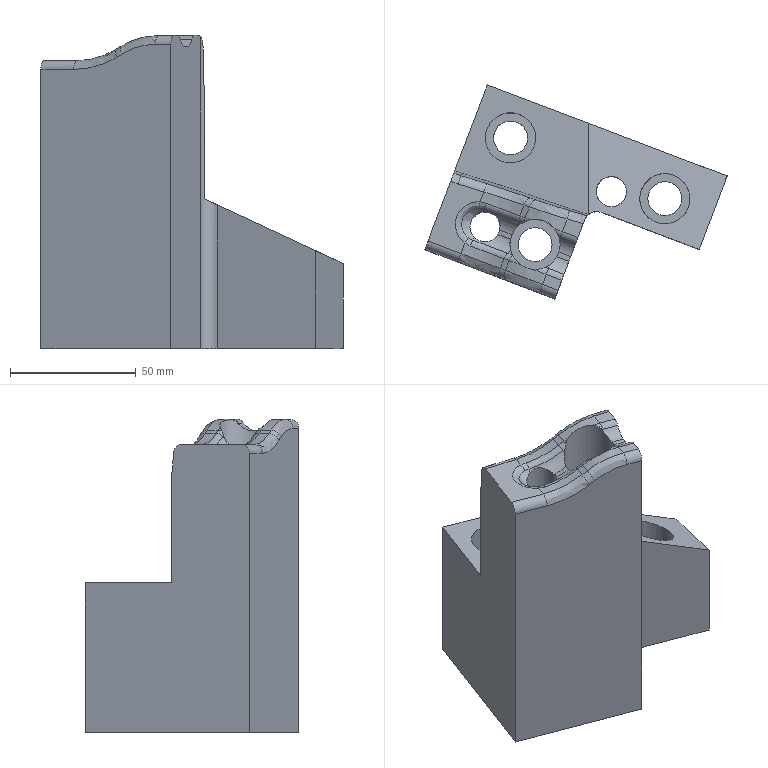Part | NX | features 23 2 | 1 solid | 68 faces | box 120.187 x 85.035 x 124.5 mm | volume 332501 mm3 | cylinder 25 | plane 18 | spline 15 | torus 10 | commonest cylinder face diameters 6 x4 13 x4 7 x3 13.5 x3 20 x3 12.001 x2